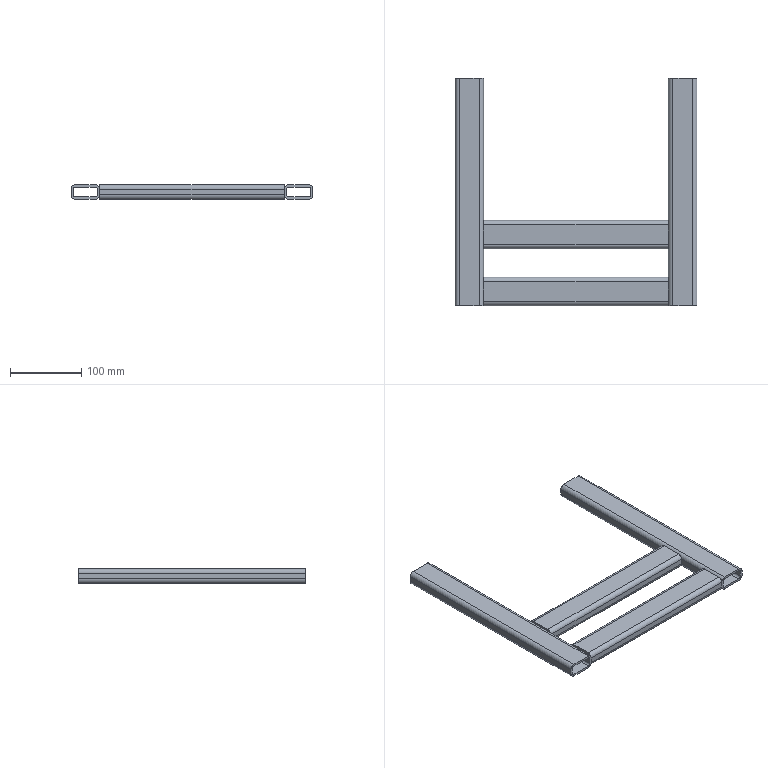Part | SolidWorks | features 3DProfileFeature 1, WeldMemberFeat 1, WeldmentFeature 1 | 4 solids | 72 faces | box 340 x 320 x 20 mm | volume 348955 mm3 | plane 40 | cylinder 32 | commonest cylinder face diameters 6 x16 12 x16